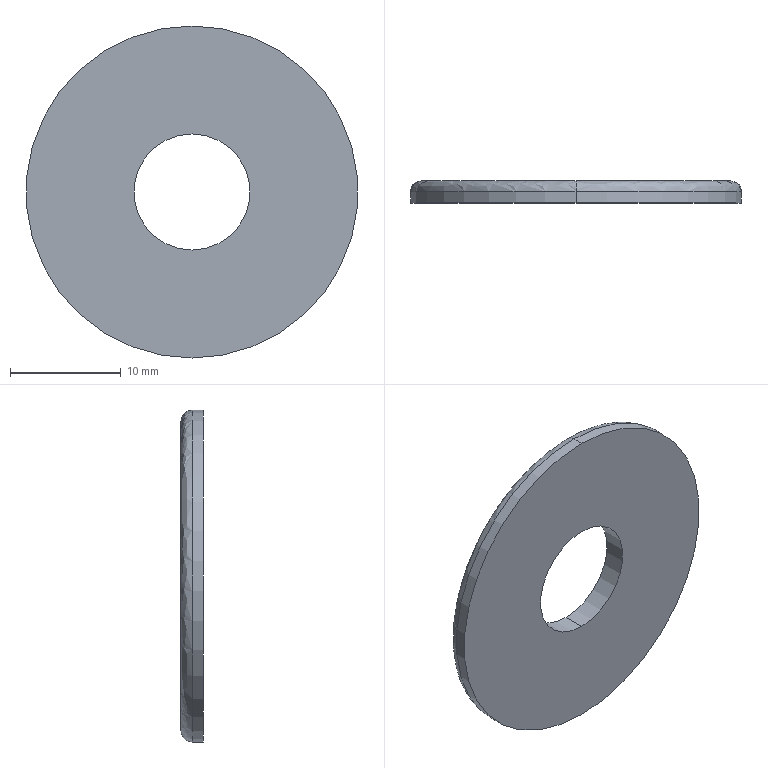Part | SolidWorks | features BaseBody 1 | 1 solid | 8 faces | box 30 x 2 x 30 mm | volume 1220 mm3 | cylinder 4 | spline 2 | plane 2 | commonest cylinder face diameters 10.5 x2 30 x2
STEP:
#1=CARTESIAN_POINT('',(0.,2.,-14.));
#2=VERTEX_POINT('',#1);
#3=CARTESIAN_POINT('',(0.,2.,14.));
#4=VERTEX_POINT('',#3);
#5=CARTESIAN_POINT('',(0.,2.,-14.));
#6=CARTESIAN_POINT('',(-0.4281,2.,-14.));
#7=CARTESIAN_POINT('',(-1.068,2.,-13.971));
#8=CARTESIAN_POINT('',(-1.809,2.,-13.886));
#9=CARTESIAN_POINT('',(-2.179,2.,-13.83));
#10=CARTESIAN_POINT('',(-2.363,2.,-13.799));
#11=CARTESIAN_POINT('',(-2.442,2.,-13.785));
#12=CARTESIAN_POINT('',(-2.495,2.,-13.776));
#13=CARTESIAN_POINT('',(-2.52,2.,-13.771));
#14=CARTESIAN_POINT('',(-2.994,2.,-13.684));
#15=CARTESIAN_POINT('',(-3.654,2.,-13.528));
#16=CARTESIAN_POINT('',(-4.409,2.,-13.291));
#17=CARTESIAN_POINT('',(-4.782,2.,-13.159));
#18=CARTESIAN_POINT('',(-4.968,2.,-13.089));
#19=CARTESIAN_POINT('',(-5.048,2.,-13.058));
#20=CARTESIAN_POINT('',(-5.101,2.,-13.038));
#21=CARTESIAN_POINT('',(-5.126,2.,-13.028));
#22=CARTESIAN_POINT('',(-5.593,2.,-12.843));
#23=CARTESIAN_POINT('',(-6.236,2.,-12.55));
#24=CARTESIAN_POINT('',(-6.958,2.,-12.153));
#25=CARTESIAN_POINT('',(-7.312,2.,-11.94));
#26=CARTESIAN_POINT('',(-7.462,2.,-11.846));
#27=CARTESIAN_POINT('',(-7.562,2.,-11.782));
#28=CARTESIAN_POINT('',(-7.61,2.,-11.751));
#29=CARTESIAN_POINT('',(-8.47,2.,-11.189));
#30=CARTESIAN_POINT('',(-9.216,2.,-10.583));
#31=CARTESIAN_POINT('',(-10.241,2.,-9.558));
#32=CARTESIAN_POINT('',(-10.725,2.,-9.022));
#33=CARTESIAN_POINT('',(-11.238,2.,-8.355));
#34=CARTESIAN_POINT('',(-11.482,2.,-8.012));
#35=CARTESIAN_POINT('',(-11.584,2.,-7.862));
#36=CARTESIAN_POINT('',(-11.651,2.,-7.762));
#37=CARTESIAN_POINT('',(-11.686,2.,-7.71));
#38=CARTESIAN_POINT('',(-11.977,2.,-7.265));
#39=CARTESIAN_POINT('',(-12.333,2.,-6.655));
#40=CARTESIAN_POINT('',(-12.694,2.,-5.914));
#41=CARTESIAN_POINT('',(-12.86,2.,-5.536));
#42=CARTESIAN_POINT('',(-12.94,2.,-5.345));
#43=CARTESIAN_POINT('',(-12.973,2.,-5.263));
#44=CARTESIAN_POINT('',(-12.995,2.,-5.208));
#45=CARTESIAN_POINT('',(-13.007,2.,-5.18));
#46=CARTESIAN_POINT('',(-13.184,2.,-4.731));
#47=CARTESIAN_POINT('',(-13.403,2.,-4.089));
#48=CARTESIAN_POINT('',(-13.603,2.,-3.324));
#49=CARTESIAN_POINT('',(-13.689,2.,-2.937));
#50=CARTESIAN_POINT('',(-13.729,2.,-2.743));
#51=CARTESIAN_POINT('',(-13.745,2.,-2.659));
#52=CARTESIAN_POINT('',(-13.756,2.,-2.603));
#53=CARTESIAN_POINT('',(-13.761,2.,-2.574));
#54=CARTESIAN_POINT('',(-13.922,2.,-1.706));
#55=CARTESIAN_POINT('',(-14.,2.,-0.856));
#56=CARTESIAN_POINT('',(-14.,2.,0.428));
#57=CARTESIAN_POINT('',(-13.971,2.,1.067));
#58=CARTESIAN_POINT('',(-13.886,2.,1.809));
#59=CARTESIAN_POINT('',(-13.83,2.,2.179));
#60=CARTESIAN_POINT('',(-13.799,2.,2.363));
#61=CARTESIAN_POINT('',(-13.785,2.,2.442));
#62=CARTESIAN_POINT('',(-13.776,2.,2.495));
#63=CARTESIAN_POINT('',(-13.771,2.,2.52));
#64=CARTESIAN_POINT('',(-13.684,2.,2.994));
#65=CARTESIAN_POINT('',(-13.528,2.,3.654));
#66=CARTESIAN_POINT('',(-13.291,2.,4.409));
#67=CARTESIAN_POINT('',(-13.159,2.,4.782));
#68=CARTESIAN_POINT('',(-13.089,2.,4.968));
#69=CARTESIAN_POINT('',(-13.058,2.,5.048));
#70=CARTESIAN_POINT('',(-13.038,2.,5.101));
#71=CARTESIAN_POINT('',(-13.028,2.,5.126));
#72=CARTESIAN_POINT('',(-12.843,2.,5.593));
#73=CARTESIAN_POINT('',(-12.55,2.,6.236));
#74=CARTESIAN_POINT('',(-12.153,2.,6.958));
#75=CARTESIAN_POINT('',(-11.94,2.,7.312));
#76=CARTESIAN_POINT('',(-11.846,2.,7.462));
#77=CARTESIAN_POINT('',(-11.782,2.,7.562));
#78=CARTESIAN_POINT('',(-11.751,2.,7.61));
#79=CARTESIAN_POINT('',(-11.189,2.,8.47));
#80=CARTESIAN_POINT('',(-10.583,2.,9.216));
#81=CARTESIAN_POINT('',(-9.558,2.,10.241));
#82=CARTESIAN_POINT('',(-9.022,2.,10.725));
#83=CARTESIAN_POINT('',(-8.355,2.,11.238));
#84=CARTESIAN_POINT('',(-8.012,2.,11.482));
#85=CARTESIAN_POINT('',(-7.862,2.,11.584));
#86=CARTESIAN_POINT('',(-7.762,2.,11.651));
#87=CARTESIAN_POINT('',(-7.71,2.,11.686));
#88=CARTESIAN_POINT('',(-7.265,2.,11.977));
#89=CARTESIAN_POINT('',(-6.655,2.,12.333));
#90=CARTESIAN_POINT('',(-5.914,2.,12.694));
#91=CARTESIAN_POINT('',(-5.536,2.,12.86));
#92=CARTESIAN_POINT('',(-5.345,2.,12.94));
#93=CARTESIAN_POINT('',(-5.263,2.,12.973));
#94=CARTESIAN_POINT('',(-5.208,2.,12.995));
#95=CARTESIAN_POINT('',(-5.18,2.,13.007));
#96=CARTESIAN_POINT('',(-4.731,2.,13.184));
#97=CARTESIAN_POINT('',(-4.089,2.,13.403));
#98=CARTESIAN_POINT('',(-3.324,2.,13.603));
#99=CARTESIAN_POINT('',(-2.937,2.,13.689));
#100=CARTESIAN_POINT('',(-2.743,2.,13.729));
#101=CARTESIAN_POINT('',(-2.659,2.,13.745));
#102=CARTESIAN_POINT('',(-2.603,2.,13.756));
#103=CARTESIAN_POINT('',(-2.574,2.,13.761));
#104=CARTESIAN_POINT('',(-1.706,2.,13.922));
#105=CARTESIAN_POINT('',(-0.8565,2.,14.));
#106=CARTESIAN_POINT('',(0.,2.,14.));
#107=B_SPLINE_CURVE_WITH_KNOTS('',3,(#5,#6,#7,#8,#9,#10,#11,#12,#13,#14,#15,#16,#17,#18,#19,#20,#21,#22,#23,#24,#25,#26,#27,#28,#29,#30,#31,#32,#33,#34,#35,#36,#37,#38,#39,#40,#41,#42,#43,#44,#45,#46,#47,#48,#49,#50,#51,#52,#53,#54,#55,#56,#57,#58,#59,#60,#61,#62,#63,#64,#65,#66,#67,#68,#69,#70,#71,#72,#73,#74,#75,#76,#77,#78,#79,#80,#81,#82,#83,#84,#85,#86,#87,#88,#89,#90,#91,#92,#93,#94,#95,#96,#97,#98,#99,#100,#101,#102,#103,#104,#105,#106),.UNSPECIFIED.,.F.,.F.,(4,1,1,1,1,2,2,1,1,1,1,2,2,1,1,1,2,2,2,1,1,1,2,2,1,1,1,1,2,2,1,1,1,1,2,2,2,1,1,1,1,2,2,1,1,1,1,2,2,1,1,1,2,2,2,1,1,1,2,2,1,1,1,1,2,2,1,1,1,1,2,2,4),(0.,0.03125,0.04687,0.05469,0.05859,0.06055,0.0625,0.09375,0.1094,0.1172,0.1211,0.123,0.125,0.1562,0.1719,0.1797,0.1836,0.1875,0.25,0.2813,0.2969,0.3047,0.3086,0.3125,0.3438,0.3594,0.3672,0.3711,0.373,0.375,0.4063,0.4219,0.4297,0.4336,0.4355,0.4375,0.5,0.5313,0.5469,0.5547,0.5586,0.5605,0.5625,0.5937,0.6094,0.6172,0.6211,0.623,0.625,0.6562,0.6719,0.6797,0.6836,0.6875,0.75,0.7812,0.7969,0.8047,0.8086,0.8125,0.8438,0.8594,0.8672,0.8711,0.873,0.875,0.9063,0.9219,0.9297,0.9336,0.9355,0.9375,1.),.UNSPECIFIED.);
#108=EDGE_CURVE('',#2,#4,#107,.T.);
#109=ORIENTED_EDGE('',*,*,#108,.F.);
#110=CARTESIAN_POINT('',(0.,1.,-15.));
#111=VERTEX_POINT('',#110);
#112=CARTESIAN_POINT('',(0.,1.,-14.));
#113=DIRECTION('',(-1.,0.,0.));
#114=DIRECTION('',(0.,0.,-1.));
#115=AXIS2_PLACEMENT_3D('',#112,#113,#114);
#116=CIRCLE('',#115,1.);
#117=EDGE_CURVE('',#2,#111,#116,.T.);
#118=ORIENTED_EDGE('',*,*,#117,.T.);
#119=CARTESIAN_POINT('',(0.,1.,15.));
#120=VERTEX_POINT('',#119);
#121=CARTESIAN_POINT('',(0.,1.,0.));
#122=DIRECTION('',(0.,-1.,0.));
#123=DIRECTION('',(0.,0.,-1.));
#124=AXIS2_PLACEMENT_3D('',#121,#122,#123);
#125=CIRCLE('',#124,15.);
#126=EDGE_CURVE('',#120,#111,#125,.T.);
#127=ORIENTED_EDGE('',*,*,#126,.F.);
#128=CARTESIAN_POINT('',(0.,1.,14.));
#129=DIRECTION('',(1.,0.,0.));
#130=DIRECTION('',(0.,0.,1.));
#131=AXIS2_PLACEMENT_3D('',#128,#129,#130);
#132=CIRCLE('',#131,1.);
#133=EDGE_CURVE('',#4,#120,#132,.T.);
#134=ORIENTED_EDGE('',*,*,#133,.F.);
#135=EDGE_LOOP('',(#109,#118,#127,#134));
#136=FACE_OUTER_BOUND('',#135,.T.);
#137=CARTESIAN_POINT('',(0.,2.,-14.));
#138=CARTESIAN_POINT('',(-28.,2.,-14.));
#139=CARTESIAN_POINT('',(-28.,2.,14.));
#140=CARTESIAN_POINT('',(0.,2.,14.));
#141=CARTESIAN_POINT('',(0.,2.,-14.586));
#142=CARTESIAN_POINT('',(-29.172,2.,-14.586));
#143=CARTESIAN_POINT('',(-29.172,2.,14.586));
#144=CARTESIAN_POINT('',(0.,2.,14.586));
#145=CARTESIAN_POINT('',(0.,1.586,-15.));
#146=CARTESIAN_POINT('',(-30.,1.586,-15.));
#147=CARTESIAN_POINT('',(-30.,1.586,15.));
#148=CARTESIAN_POINT('',(0.,1.586,15.));
#149=CARTESIAN_POINT('',(0.,1.,-15.));
#150=CARTESIAN_POINT('',(-30.,1.,-15.));
#151=CARTESIAN_POINT('',(-30.,1.,15.));
#152=CARTESIAN_POINT('',(0.,1.,15.));
#153=(BOUNDED_SURFACE()B_SPLINE_SURFACE(3,3,((#137,#138,#139,#140),(#141,#142,#143,#144),(#145,#146,#147,#148),(#149,#150,#151,#152)),.UNSPECIFIED.,.F.,.F.,.T.)B_SPLINE_SURFACE_WITH_KNOTS((4,4),(4,4),(0.,1.),(0.,1.),.UNSPECIFIED.)GEOMETRIC_REPRESENTATION_ITEM()RATIONAL_B_SPLINE_SURFACE(((1.,0.3333,0.3333,1.),(0.8047,0.2682,0.2682,0.8047),(0.8047,0.2682,0.2682,0.8047),(1.,0.3333,0.3333,1.)))REPRESENTATION_ITEM('')SURFACE());
#154=ADVANCED_FACE('',(#136),#153,.T.);
#155=CARTESIAN_POINT('',(0.,0.,5.25));
#156=VERTEX_POINT('',#155);
#157=CARTESIAN_POINT('',(0.,0.,-5.25));
#158=VERTEX_POINT('',#157);
#159=CARTESIAN_POINT('',(0.,0.,0.));
#160=DIRECTION('',(0.,-1.,0.));
#161=DIRECTION('',(0.,0.,1.));
#162=AXIS2_PLACEMENT_3D('',#159,#160,#161);
#163=CIRCLE('',#162,5.25);
#164=EDGE_CURVE('',#156,#158,#163,.T.);
#165=ORIENTED_EDGE('',*,*,#164,.T.);
#166=CARTESIAN_POINT('',(0.,2.,-5.25));
#167=VERTEX_POINT('',#166);
#168=CARTESIAN_POINT('',(0.,0.,-5.25));
#169=DIRECTION('',(0.,1.,0.));
#170=VECTOR('',#169,1000.);
#171=LINE('',#168,#170);
#172=EDGE_CURVE('',#158,#167,#171,.T.);
#173=ORIENTED_EDGE('',*,*,#172,.T.);
#174=CARTESIAN_POINT('',(0.,2.,5.25));
#175=VERTEX_POINT('',#174);
#176=CARTESIAN_POINT('',(0.,2.,0.));
#177=DIRECTION('',(0.,-1.,0.));
#178=DIRECTION('',(0.,0.,1.));
#179=AXIS2_PLACEMENT_3D('',#176,#177,#178);
#180=CIRCLE('',#179,5.25);
#181=EDGE_CURVE('',#175,#167,#180,.T.);
#182=ORIENTED_EDGE('',*,*,#181,.F.);
#183=CARTESIAN_POINT('',(0.,0.,5.25));
#184=DIRECTION('',(0.,1.,0.));
#185=VECTOR('',#184,1000.);
#186=LINE('',#183,#185);
#187=EDGE_CURVE('',#156,#175,#186,.T.);
#188=ORIENTED_EDGE('',*,*,#187,.F.);
#189=EDGE_LOOP('',(#165,#173,#182,#188));
#190=FACE_OUTER_BOUND('',#189,.T.);
#191=CARTESIAN_POINT('',(0.,0.,0.));
#192=DIRECTION('',(0.,1.,0.));
#193=DIRECTION('',(0.,0.,1.));
#194=AXIS2_PLACEMENT_3D('',#191,#192,#193);
#195=CYLINDRICAL_SURFACE('',#194,5.25);
#196=ADVANCED_FACE('',(#190),#195,.F.);
#197=CARTESIAN_POINT('',(0.,1.,0.));
#198=DIRECTION('',(0.,-1.,0.));
#199=DIRECTION('',(0.,0.,-1.));
#200=AXIS2_PLACEMENT_3D('',#197,#198,#199);
#201=CIRCLE('',#200,15.);
#202=EDGE_CURVE('',#111,#120,#201,.T.);
#203=ORIENTED_EDGE('',*,*,#202,.T.);
#204=CARTESIAN_POINT('',(0.,0.,15.));
#205=VERTEX_POINT('',#204);
#206=CARTESIAN_POINT('',(0.,2.,15.));
#207=DIRECTION('',(0.,-1.,0.));
#208=VECTOR('',#207,1000.);
#209=LINE('',#206,#208);
#210=EDGE_CURVE('',#120,#205,#209,.T.);
#211=ORIENTED_EDGE('',*,*,#210,.T.);
#212=CARTESIAN_POINT('',(0.,0.,-15.));
#213=VERTEX_POINT('',#212);
#214=CARTESIAN_POINT('',(0.,0.,0.));
#215=DIRECTION('',(0.,1.,0.));
#216=DIRECTION('',(0.,0.,-1.));
#217=AXIS2_PLACEMENT_3D('',#214,#215,#216);
#218=CIRCLE('',#217,15.);
#219=EDGE_CURVE('',#205,#213,#218,.T.);
#220=ORIENTED_EDGE('',*,*,#219,.T.);
#221=CARTESIAN_POINT('',(0.,2.,-15.));
#222=DIRECTION('',(0.,-1.,0.));
#223=VECTOR('',#222,1000.);
#224=LINE('',#221,#223);
#225=EDGE_CURVE('',#111,#213,#224,.T.);
#226=ORIENTED_EDGE('',*,*,#225,.F.);
#227=EDGE_LOOP('',(#203,#211,#220,#226));
#228=FACE_OUTER_BOUND('',#227,.T.);
#229=CARTESIAN_POINT('',(0.,2.,0.));
#230=DIRECTION('',(0.,-1.,0.));
#231=DIRECTION('',(0.,0.,-1.));
#232=AXIS2_PLACEMENT_3D('',#229,#230,#231);
#233=CYLINDRICAL_SURFACE('',#232,15.);
#234=ADVANCED_FACE('',(#228),#233,.T.);
#235=ORIENTED_EDGE('',*,*,#164,.F.);
#236=CARTESIAN_POINT('',(0.,0.,0.));
#237=DIRECTION('',(0.,-1.,0.));
#238=DIRECTION('',(0.,0.,1.));
#239=AXIS2_PLACEMENT_3D('',#236,#237,#238);
#240=CIRCLE('',#239,5.25);
#241=EDGE_CURVE('',#158,#156,#240,.T.);
#242=ORIENTED_EDGE('',*,*,#241,.F.);
#243=EDGE_LOOP('',(#235,#242));
#244=FACE_BOUND('',#243,.T.);
#245=CARTESIAN_POINT('',(0.,0.,0.));
#246=DIRECTION('',(0.,1.,0.));
#247=DIRECTION('',(0.,0.,-1.));
#248=AXIS2_PLACEMENT_3D('',#245,#246,#247);
#249=CIRCLE('',#248,15.);
#250=EDGE_CURVE('',#213,#205,#249,.T.);
#251=ORIENTED_EDGE('',*,*,#250,.F.);
#252=ORIENTED_EDGE('',*,*,#219,.F.);
#253=EDGE_LOOP('',(#251,#252));
#254=FACE_OUTER_BOUND('',#253,.T.);
#255=CARTESIAN_POINT('',(0.,0.,0.));
#256=DIRECTION('',(0.,1.,0.));
#257=DIRECTION('',(0.,0.,1.));
#258=AXIS2_PLACEMENT_3D('',#255,#256,#257);
#259=PLANE('',#258);
#260=ADVANCED_FACE('',(#244,#254),#259,.F.);
#261=ORIENTED_EDGE('',*,*,#172,.F.);
#262=ORIENTED_EDGE('',*,*,#241,.T.);
#263=ORIENTED_EDGE('',*,*,#187,.T.);
#264=CARTESIAN_POINT('',(0.,2.,0.));
#265=DIRECTION('',(0.,-1.,0.));
#266=DIRECTION('',(0.,0.,1.));
#267=AXIS2_PLACEMENT_3D('',#264,#265,#266);
#268=CIRCLE('',#267,5.25);
#269=EDGE_CURVE('',#167,#175,#268,.T.);
#270=ORIENTED_EDGE('',*,*,#269,.F.);
#271=EDGE_LOOP('',(#261,#262,#263,#270));
#272=FACE_OUTER_BOUND('',#271,.T.);
#273=CARTESIAN_POINT('',(0.,0.,0.));
#274=DIRECTION('',(0.,1.,0.));
#275=DIRECTION('',(0.,0.,1.));
#276=AXIS2_PLACEMENT_3D('',#273,#274,#275);
#277=CYLINDRICAL_SURFACE('',#276,5.25);
#278=ADVANCED_FACE('',(#272),#277,.F.);
#279=ORIENTED_EDGE('',*,*,#210,.F.);
#280=ORIENTED_EDGE('',*,*,#126,.T.);
#281=ORIENTED_EDGE('',*,*,#225,.T.);
#282=ORIENTED_EDGE('',*,*,#250,.T.);
#283=EDGE_LOOP('',(#279,#280,#281,#282));
#284=FACE_OUTER_BOUND('',#283,.T.);
#285=CARTESIAN_POINT('',(0.,2.,0.));
#286=DIRECTION('',(0.,-1.,0.));
#287=DIRECTION('',(0.,0.,-1.));
#288=AXIS2_PLACEMENT_3D('',#285,#286,#287);
#289=CYLINDRICAL_SURFACE('',#288,15.);
#290=ADVANCED_FACE('',(#284),#289,.T.);
#291=ORIENTED_EDGE('',*,*,#181,.T.);
#292=ORIENTED_EDGE('',*,*,#269,.T.);
#293=EDGE_LOOP('',(#291,#292));
#294=FACE_BOUND('',#293,.T.);
#295=CARTESIAN_POINT('',(0.,2.,14.));
#296=CARTESIAN_POINT('',(0.4281,2.,14.));
#297=CARTESIAN_POINT('',(1.068,2.,13.971));
#298=CARTESIAN_POINT('',(1.809,2.,13.886));
#299=CARTESIAN_POINT('',(2.179,2.,13.83));
#300=CARTESIAN_POINT('',(2.363,2.,13.799));
#301=CARTESIAN_POINT('',(2.442,2.,13.785));
#302=CARTESIAN_POINT('',(2.495,2.,13.776));
#303=CARTESIAN_POINT('',(2.52,2.,13.771));
#304=CARTESIAN_POINT('',(2.994,2.,13.684));
#305=CARTESIAN_POINT('',(3.654,2.,13.528));
#306=CARTESIAN_POINT('',(4.409,2.,13.291));
#307=CARTESIAN_POINT('',(4.782,2.,13.159));
#308=CARTESIAN_POINT('',(4.968,2.,13.089));
#309=CARTESIAN_POINT('',(5.048,2.,13.058));
#310=CARTESIAN_POINT('',(5.101,2.,13.038));
#311=CARTESIAN_POINT('',(5.126,2.,13.028));
#312=CARTESIAN_POINT('',(5.593,2.,12.843));
#313=CARTESIAN_POINT('',(6.236,2.,12.55));
#314=CARTESIAN_POINT('',(6.958,2.,12.153));
#315=CARTESIAN_POINT('',(7.312,2.,11.94));
#316=CARTESIAN_POINT('',(7.462,2.,11.846));
#317=CARTESIAN_POINT('',(7.562,2.,11.782));
#318=CARTESIAN_POINT('',(7.61,2.,11.751));
#319=CARTESIAN_POINT('',(8.47,2.,11.189));
#320=CARTESIAN_POINT('',(9.216,2.,10.583));
#321=CARTESIAN_POINT('',(10.241,2.,9.558));
#322=CARTESIAN_POINT('',(10.725,2.,9.022));
#323=CARTESIAN_POINT('',(11.238,2.,8.355));
#324=CARTESIAN_POINT('',(11.482,2.,8.012));
#325=CARTESIAN_POINT('',(11.584,2.,7.862));
#326=CARTESIAN_POINT('',(11.651,2.,7.762));
#327=CARTESIAN_POINT('',(11.686,2.,7.71));
#328=CARTESIAN_POINT('',(11.977,2.,7.265));
#329=CARTESIAN_POINT('',(12.333,2.,6.655));
#330=CARTESIAN_POINT('',(12.694,2.,5.914));
#331=CARTESIAN_POINT('',(12.86,2.,5.536));
#332=CARTESIAN_POINT('',(12.94,2.,5.345));
#333=CARTESIAN_POINT('',(12.973,2.,5.263));
#334=CARTESIAN_POINT('',(12.995,2.,5.208));
#335=CARTESIAN_POINT('',(13.007,2.,5.18));
#336=CARTESIAN_POINT('',(13.184,2.,4.731));
#337=CARTESIAN_POINT('',(13.403,2.,4.089));
#338=CARTESIAN_POINT('',(13.603,2.,3.324));
#339=CARTESIAN_POINT('',(13.689,2.,2.937));
#340=CARTESIAN_POINT('',(13.729,2.,2.743));
#341=CARTESIAN_POINT('',(13.745,2.,2.659));
#342=CARTESIAN_POINT('',(13.756,2.,2.603));
#343=CARTESIAN_POINT('',(13.761,2.,2.574));
#344=CARTESIAN_POINT('',(13.922,2.,1.706));
#345=CARTESIAN_POINT('',(14.,2.,0.856));
#346=CARTESIAN_POINT('',(14.,2.,-0.428));
#347=CARTESIAN_POINT('',(13.971,2.,-1.067));
#348=CARTESIAN_POINT('',(13.886,2.,-1.809));
#349=CARTESIAN_POINT('',(13.83,2.,-2.179));
#350=CARTESIAN_POINT('',(13.799,2.,-2.363));
#351=CARTESIAN_POINT('',(13.785,2.,-2.442));
#352=CARTESIAN_POINT('',(13.776,2.,-2.495));
#353=CARTESIAN_POINT('',(13.771,2.,-2.52));
#354=CARTESIAN_POINT('',(13.684,2.,-2.994));
#355=CARTESIAN_POINT('',(13.528,2.,-3.654));
#356=CARTESIAN_POINT('',(13.291,2.,-4.409));
#357=CARTESIAN_POINT('',(13.159,2.,-4.782));
#358=CARTESIAN_POINT('',(13.089,2.,-4.968));
#359=CARTESIAN_POINT('',(13.058,2.,-5.048));
#360=CARTESIAN_POINT('',(13.038,2.,-5.101));
#361=CARTESIAN_POINT('',(13.028,2.,-5.126));
#362=CARTESIAN_POINT('',(12.843,2.,-5.593));
#363=CARTESIAN_POINT('',(12.55,2.,-6.236));
#364=CARTESIAN_POINT('',(12.153,2.,-6.958));
#365=CARTESIAN_POINT('',(11.94,2.,-7.312));
#366=CARTESIAN_POINT('',(11.846,2.,-7.462));
#367=CARTESIAN_POINT('',(11.782,2.,-7.562));
#368=CARTESIAN_POINT('',(11.751,2.,-7.61));
#369=CARTESIAN_POINT('',(11.189,2.,-8.47));
#370=CARTESIAN_POINT('',(10.583,2.,-9.216));
#371=CARTESIAN_POINT('',(9.558,2.,-10.241));
#372=CARTESIAN_POINT('',(9.022,2.,-10.725));
#373=CARTESIAN_POINT('',(8.355,2.,-11.238));
#374=CARTESIAN_POINT('',(8.012,2.,-11.482));
#375=CARTESIAN_POINT('',(7.862,2.,-11.584));
#376=CARTESIAN_POINT('',(7.762,2.,-11.651));
#377=CARTESIAN_POINT('',(7.71,2.,-11.686));
#378=CARTESIAN_POINT('',(7.265,2.,-11.977));
#379=CARTESIAN_POINT('',(6.655,2.,-12.333));
#380=CARTESIAN_POINT('',(5.914,2.,-12.694));
#381=CARTESIAN_POINT('',(5.536,2.,-12.86));
#382=CARTESIAN_POINT('',(5.345,2.,-12.94));
#383=CARTESIAN_POINT('',(5.263,2.,-12.973));
#384=CARTESIAN_POINT('',(5.208,2.,-12.995));
#385=CARTESIAN_POINT('',(5.18,2.,-13.007));
#386=CARTESIAN_POINT('',(4.731,2.,-13.184));
#387=CARTESIAN_POINT('',(4.089,2.,-13.403));
#388=CARTESIAN_POINT('',(3.324,2.,-13.603));
#389=CARTESIAN_POINT('',(2.937,2.,-13.689));
#390=CARTESIAN_POINT('',(2.743,2.,-13.729));
#391=CARTESIAN_POINT('',(2.659,2.,-13.745));
#392=CARTESIAN_POINT('',(2.603,2.,-13.756));
#393=CARTESIAN_POINT('',(2.574,2.,-13.761));
#394=CARTESIAN_POINT('',(1.706,2.,-13.922));
#395=CARTESIAN_POINT('',(0.8565,2.,-14.));
#396=CARTESIAN_POINT('',(0.,2.,-14.));
#397=B_SPLINE_CURVE_WITH_KNOTS('',3,(#295,#296,#297,#298,#299,#300,#301,#302,#303,#304,#305,#306,#307,#308,#309,#310,#311,#312,#313,#314,#315,#316,#317,#318,#319,#320,#321,#322,#323,#324,#325,#326,#327,#328,#329,#330,#331,#332,#333,#334,#335,#336,#337,#338,#339,#340,#341,#342,#343,#344,#345,#346,#347,#348,#349,#350,#351,#352,#353,#354,#355,#356,#357,#358,#359,#360,#361,#362,#363,#364,#365,#366,#367,#368,#369,#370,#371,#372,#373,#374,#375,#376,#377,#378,#379,#380,#381,#382,#383,#384,#385,#386,#387,#388,#389,#390,#391,#392,#393,#394,#395,#396),.UNSPECIFIED.,.F.,.F.,(4,1,1,1,1,2,2,1,1,1,1,2,2,1,1,1,2,2,2,1,1,1,2,2,1,1,1,1,2,2,1,1,1,1,2,2,2,1,1,1,1,2,2,1,1,1,1,2,2,1,1,1,2,2,2,1,1,1,2,2,1,1,1,1,2,2,1,1,1,1,2,2,4),(0.,0.03125,0.04687,0.05469,0.05859,0.06055,0.0625,0.09375,0.1094,0.1172,0.1211,0.123,0.125,0.1562,0.1719,0.1797,0.1836,0.1875,0.25,0.2812,0.2969,0.3047,0.3086,0.3125,0.3437,0.3594,0.3672,0.3711,0.373,0.375,0.4062,0.4219,0.4297,0.4336,0.4355,0.4375,0.5,0.5312,0.5469,0.5547,0.5586,0.5605,0.5625,0.5937,0.6094,0.6172,0.6211,0.623,0.625,0.6562,0.6719,0.6797,0.6836,0.6875,0.75,0.7812,0.7969,0.8047,0.8086,0.8125,0.8437,0.8594,0.8672,0.8711,0.873,0.875,0.9062,0.9219,0.9297,0.9336,0.9355,0.9375,1.),.UNSPECIFIED.);
#398=EDGE_CURVE('',#4,#2,#397,.T.);
#399=ORIENTED_EDGE('',*,*,#398,.T.);
#400=ORIENTED_EDGE('',*,*,#108,.T.);
#401=EDGE_LOOP('',(#399,#400));
#402=FACE_OUTER_BOUND('',#401,.T.);
#403=CARTESIAN_POINT('',(0.,2.,0.));
#404=DIRECTION('',(0.,1.,0.));
#405=DIRECTION('',(0.,0.,1.));
#406=AXIS2_PLACEMENT_3D('',#403,#404,#405);
#407=PLANE('',#406);
#408=ADVANCED_FACE('',(#294,#402),#407,.T.);
#409=ORIENTED_EDGE('',*,*,#117,.F.);
#410=ORIENTED_EDGE('',*,*,#398,.F.);
#411=ORIENTED_EDGE('',*,*,#133,.T.);
#412=ORIENTED_EDGE('',*,*,#202,.F.);
#413=EDGE_LOOP('',(#409,#410,#411,#412));
#414=FACE_OUTER_BOUND('',#413,.T.);
#415=CARTESIAN_POINT('',(0.,2.,14.));
#416=CARTESIAN_POINT('',(28.,2.,14.));
#417=CARTESIAN_POINT('',(28.,2.,-14.));
#418=CARTESIAN_POINT('',(0.,2.,-14.));
#419=CARTESIAN_POINT('',(0.,2.,14.586));
#420=CARTESIAN_POINT('',(29.172,2.,14.586));
#421=CARTESIAN_POINT('',(29.172,2.,-14.586));
#422=CARTESIAN_POINT('',(0.,2.,-14.586));
#423=CARTESIAN_POINT('',(0.,1.586,15.));
#424=CARTESIAN_POINT('',(30.,1.586,15.));
#425=CARTESIAN_POINT('',(30.,1.586,-15.));
#426=CARTESIAN_POINT('',(0.,1.586,-15.));
#427=CARTESIAN_POINT('',(0.,1.,15.));
#428=CARTESIAN_POINT('',(30.,1.,15.));
#429=CARTESIAN_POINT('',(30.,1.,-15.));
#430=CARTESIAN_POINT('',(0.,1.,-15.));
#431=(BOUNDED_SURFACE()B_SPLINE_SURFACE(3,3,((#415,#416,#417,#418),(#419,#420,#421,#422),(#423,#424,#425,#426),(#427,#428,#429,#430)),.UNSPECIFIED.,.F.,.F.,.T.)B_SPLINE_SURFACE_WITH_KNOTS((4,4),(4,4),(0.,1.),(0.,1.),.UNSPECIFIED.)GEOMETRIC_REPRESENTATION_ITEM()RATIONAL_B_SPLINE_SURFACE(((1.,0.3333,0.3333,1.),(0.8047,0.2682,0.2682,0.8047),(0.8047,0.2682,0.2682,0.8047),(1.,0.3333,0.3333,1.)))REPRESENTATION_ITEM('')SURFACE());
#432=ADVANCED_FACE('',(#414),#431,.T.);
#433=CLOSED_SHELL('',(#154,#196,#234,#260,#278,#290,#408,#432));
#434=MANIFOLD_SOLID_BREP('',#433);
#435=CARTESIAN_POINT('',(0.,0.,0.));
#436=DIRECTION('',(0.,0.,1.));
#437=DIRECTION('',(1.,0.,0.));
#438=AXIS2_PLACEMENT_3D('',#435,#436,#437);
#439=(LENGTH_UNIT()NAMED_UNIT(*)SI_UNIT(.MILLI.,.METRE.));
#440=UNCERTAINTY_MEASURE_WITH_UNIT(LENGTH_MEASURE(0.00001),#439,'','');
#441=(NAMED_UNIT(*)PLANE_ANGLE_UNIT()SI_UNIT($,.RADIAN.));
#442=(NAMED_UNIT(*)SI_UNIT($,.STERADIAN.)SOLID_ANGLE_UNIT());
#443=(GEOMETRIC_REPRESENTATION_CONTEXT(3)GLOBAL_UNCERTAINTY_ASSIGNED_CONTEXT((#440))GLOBAL_UNIT_ASSIGNED_CONTEXT((#439,#441,#442))REPRESENTATION_CONTEXT('',''));
#444=ADVANCED_BREP_SHAPE_REPRESENTATION('',(#434,#438),#443);